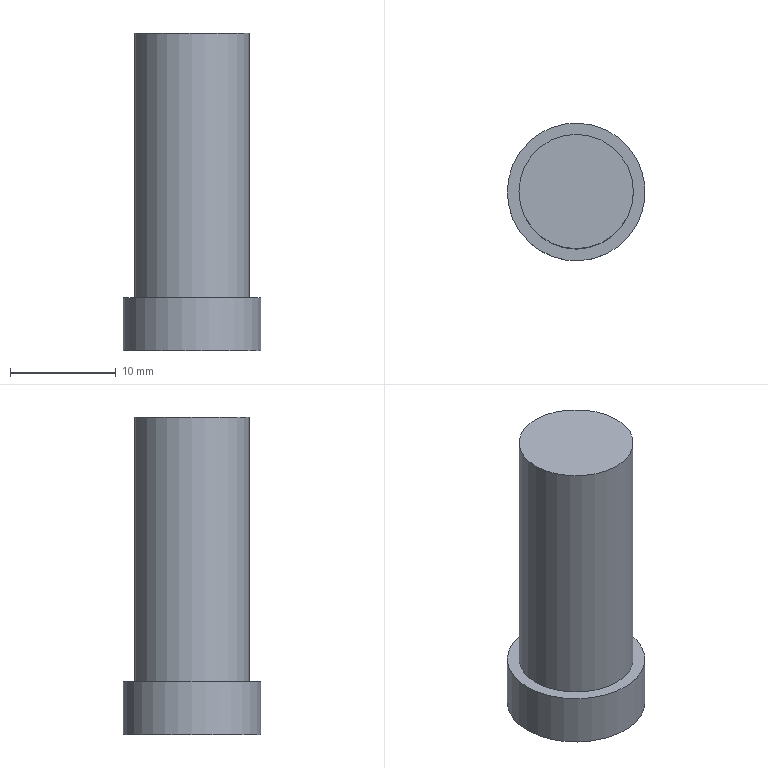Part | NX | features solid 2 | 1 solid | 5 faces | box 13 x 13 x 30 mm | volume 2954 mm3 | plane 3 | cylinder 2 | commonest cylinder face diameters 10.8 x1 13 x1
STEP:
#1=CARTESIAN_POINT('',(2464.497,-809.449,853.716));
#2=VERTEX_POINT('',#1);
#3=CARTESIAN_POINT('',(2459.097,-809.449,853.716));
#4=DIRECTION('',(0.,0.,1.));
#5=DIRECTION('',(1.,0.,0.));
#6=AXIS2_PLACEMENT_3D('',#3,#4,#5);
#7=CIRCLE('',#6,5.4);
#8=EDGE_CURVE('',#2,#2,#7,.F.);
#9=ORIENTED_EDGE('',*,*,#8,.T.);
#10=EDGE_LOOP('',(#9));
#11=FACE_BOUND('',#10,.T.);
#12=CARTESIAN_POINT('',(2453.697,-809.449,828.716));
#13=VERTEX_POINT('',#12);
#14=CARTESIAN_POINT('',(2459.097,-809.449,828.716));
#15=DIRECTION('',(0.,0.,-1.));
#16=DIRECTION('',(-1.,0.,0.));
#17=AXIS2_PLACEMENT_3D('',#14,#15,#16);
#18=CIRCLE('',#17,5.4);
#19=EDGE_CURVE('',#13,#13,#18,.T.);
#20=ORIENTED_EDGE('',*,*,#19,.F.);
#21=EDGE_LOOP('',(#20));
#22=FACE_BOUND('',#21,.T.);
#23=CARTESIAN_POINT('',(2459.097,-809.449,858.3));
#24=DIRECTION('',(0.,0.,-1.));
#25=DIRECTION('',(-1.,0.,0.));
#26=AXIS2_PLACEMENT_3D('',#23,#24,#25);
#27=CYLINDRICAL_SURFACE('',#26,5.4);
#28=ADVANCED_FACE('',(#11,#22),#27,.T.);
#29=ORIENTED_EDGE('',*,*,#8,.F.);
#30=EDGE_LOOP('',(#29));
#31=FACE_BOUND('',#30,.T.);
#32=CARTESIAN_POINT('',(2459.086,-799.952,853.716));
#33=DIRECTION('',(0.,0.,1.));
#34=DIRECTION('',(1.,0.,0.));
#35=AXIS2_PLACEMENT_3D('',#32,#33,#34);
#36=PLANE('',#35);
#37=ADVANCED_FACE('',(#31),#36,.T.);
#38=CARTESIAN_POINT('',(2452.597,-809.449,823.716));
#39=VERTEX_POINT('',#38);
#40=CARTESIAN_POINT('',(2459.097,-809.449,823.716));
#41=DIRECTION('',(0.,0.,-1.));
#42=DIRECTION('',(-1.,0.,0.));
#43=AXIS2_PLACEMENT_3D('',#40,#41,#42);
#44=CIRCLE('',#43,6.5);
#45=EDGE_CURVE('',#39,#39,#44,.F.);
#46=ORIENTED_EDGE('',*,*,#45,.F.);
#47=EDGE_LOOP('',(#46));
#48=FACE_BOUND('',#47,.T.);
#49=CARTESIAN_POINT('',(2459.097,-799.949,823.716));
#50=DIRECTION('',(0.,0.,-1.));
#51=DIRECTION('',(0.,1.,0.));
#52=AXIS2_PLACEMENT_3D('',#49,#50,#51);
#53=PLANE('',#52);
#54=ADVANCED_FACE('',(#48),#53,.T.);
#55=CARTESIAN_POINT('',(2452.597,-809.449,828.716));
#56=VERTEX_POINT('',#55);
#57=CARTESIAN_POINT('',(2459.097,-809.449,828.716));
#58=DIRECTION('',(0.,0.,-1.));
#59=DIRECTION('',(-1.,0.,0.));
#60=AXIS2_PLACEMENT_3D('',#57,#58,#59);
#61=CIRCLE('',#60,6.5);
#62=EDGE_CURVE('',#56,#56,#61,.F.);
#63=ORIENTED_EDGE('',*,*,#62,.F.);
#64=EDGE_LOOP('',(#63));
#65=FACE_BOUND('',#64,.T.);
#66=ORIENTED_EDGE('',*,*,#45,.T.);
#67=EDGE_LOOP('',(#66));
#68=FACE_BOUND('',#67,.T.);
#69=CARTESIAN_POINT('',(2459.097,-809.449,858.3));
#70=DIRECTION('',(0.,0.,-1.));
#71=DIRECTION('',(-1.,0.,0.));
#72=AXIS2_PLACEMENT_3D('',#69,#70,#71);
#73=CYLINDRICAL_SURFACE('',#72,6.5);
#74=ADVANCED_FACE('',(#65,#68),#73,.T.);
#75=ORIENTED_EDGE('',*,*,#19,.T.);
#76=EDGE_LOOP('',(#75));
#77=FACE_BOUND('',#76,.T.);
#78=ORIENTED_EDGE('',*,*,#62,.T.);
#79=EDGE_LOOP('',(#78));
#80=FACE_BOUND('',#79,.T.);
#81=CARTESIAN_POINT('',(2459.097,-809.449,828.716));
#82=DIRECTION('',(0.,0.,-1.));
#83=DIRECTION('',(-1.,0.,0.));
#84=AXIS2_PLACEMENT_3D('',#81,#82,#83);
#85=PLANE('',#84);
#86=ADVANCED_FACE('',(#77,#80),#85,.F.);
#87=CLOSED_SHELL('',(#28,#37,#54,#74,#86));
#88=MANIFOLD_SOLID_BREP('',#87);
#89=(LENGTH_UNIT()NAMED_UNIT(*)SI_UNIT(.MILLI.,.METRE.));
#90=UNCERTAINTY_MEASURE_WITH_UNIT(LENGTH_MEASURE(0.00001),#89,'','');
#91=(NAMED_UNIT(*)PLANE_ANGLE_UNIT()SI_UNIT($,.RADIAN.));
#92=(NAMED_UNIT(*)SI_UNIT($,.STERADIAN.)SOLID_ANGLE_UNIT());
#93=(GEOMETRIC_REPRESENTATION_CONTEXT(3)GLOBAL_UNCERTAINTY_ASSIGNED_CONTEXT((#90))GLOBAL_UNIT_ASSIGNED_CONTEXT((#89,#91,#92))REPRESENTATION_CONTEXT('',''));
#94=ADVANCED_BREP_SHAPE_REPRESENTATION('',(#88),#93);